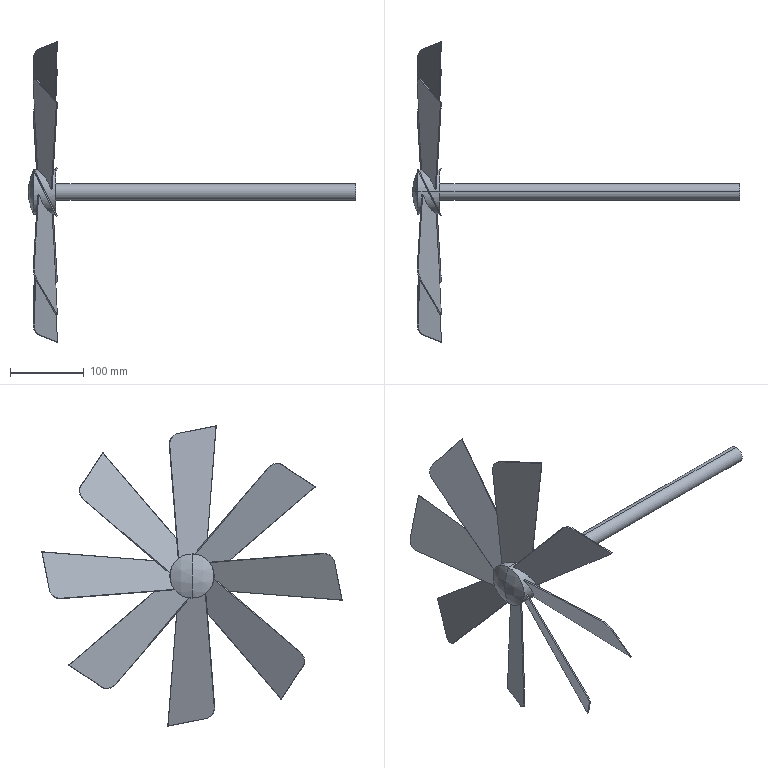Part | SolidWorks | features ICE 9, Revolution 3, CirPattern 2, Cut 1, Helix 1, RefAxis 1, Scale 1, SweepCut 1 | 1 solid | 66 faces | box 444 x 407.086 x 407.086 mm | volume 372083 mm3 | plane 42 | cylinder 22 | sphere 2 | commonest cylinder face diameters 30 x18 22.5 x2 60 x2